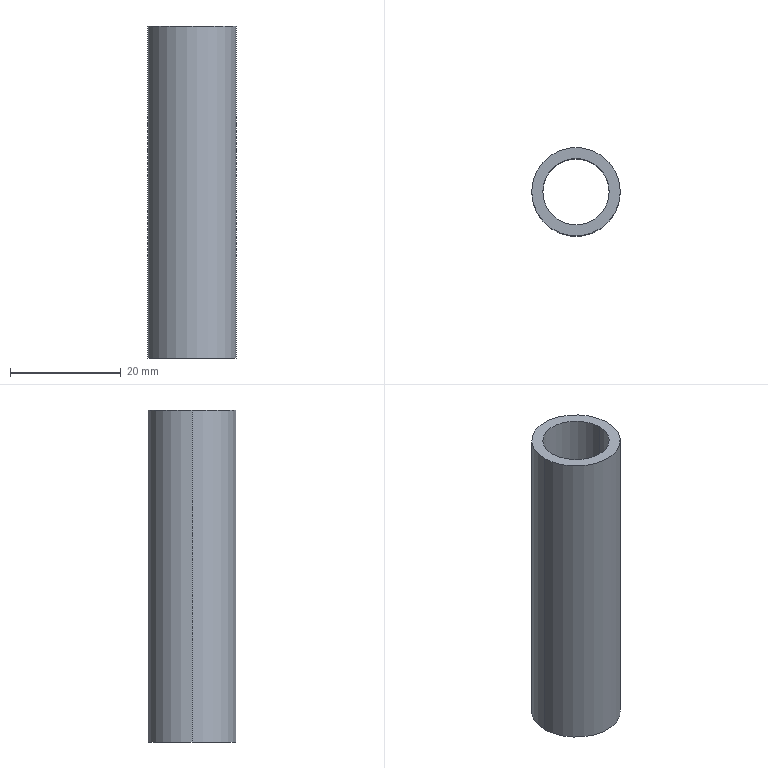Part | SolidWorks | features Extrusion 1 | 1 solid | 6 faces | box 16 x 16 x 60 mm | volume 5278 mm3 | cylinder 4 | plane 2 | commonest cylinder face diameters 12 x2 16 x2
STEP:
#1=CARTESIAN_POINT('',(-6.,0.,60.));
#2=VERTEX_POINT('',#1);
#3=CARTESIAN_POINT('',(6.,0.,60.));
#4=VERTEX_POINT('',#3);
#5=CARTESIAN_POINT('',(0.,0.,60.));
#6=DIRECTION('',(0.,0.,1.));
#7=DIRECTION('',(1.,0.,0.));
#8=AXIS2_PLACEMENT_3D('',#5,#6,#7);
#9=CIRCLE('',#8,6.);
#10=EDGE_CURVE('',#2,#4,#9,.T.);
#11=ORIENTED_EDGE('',*,*,#10,.T.);
#12=CARTESIAN_POINT('',(6.,0.,0.));
#13=VERTEX_POINT('',#12);
#14=CARTESIAN_POINT('',(6.,0.,60.));
#15=DIRECTION('',(0.,0.,-1.));
#16=VECTOR('',#15,1000.);
#17=LINE('',#14,#16);
#18=EDGE_CURVE('',#4,#13,#17,.T.);
#19=ORIENTED_EDGE('',*,*,#18,.T.);
#20=CARTESIAN_POINT('',(-6.,0.,0.));
#21=VERTEX_POINT('',#20);
#22=CARTESIAN_POINT('',(0.,0.,0.));
#23=DIRECTION('',(0.,0.,1.));
#24=DIRECTION('',(1.,0.,0.));
#25=AXIS2_PLACEMENT_3D('',#22,#23,#24);
#26=CIRCLE('',#25,6.);
#27=EDGE_CURVE('',#21,#13,#26,.T.);
#28=ORIENTED_EDGE('',*,*,#27,.F.);
#29=CARTESIAN_POINT('',(-6.,0.,60.));
#30=DIRECTION('',(0.,0.,-1.));
#31=VECTOR('',#30,1000.);
#32=LINE('',#29,#31);
#33=EDGE_CURVE('',#2,#21,#32,.T.);
#34=ORIENTED_EDGE('',*,*,#33,.F.);
#35=EDGE_LOOP('',(#11,#19,#28,#34));
#36=FACE_OUTER_BOUND('',#35,.T.);
#37=CARTESIAN_POINT('',(0.,0.,60.));
#38=DIRECTION('',(0.,0.,-1.));
#39=DIRECTION('',(-1.,0.,0.));
#40=AXIS2_PLACEMENT_3D('',#37,#38,#39);
#41=CYLINDRICAL_SURFACE('',#40,6.);
#42=ADVANCED_FACE('',(#36),#41,.F.);
#43=CARTESIAN_POINT('',(8.,0.,60.));
#44=VERTEX_POINT('',#43);
#45=CARTESIAN_POINT('',(-8.,0.,60.));
#46=VERTEX_POINT('',#45);
#47=CARTESIAN_POINT('',(0.,0.,60.));
#48=DIRECTION('',(0.,0.,1.));
#49=DIRECTION('',(1.,0.,0.));
#50=AXIS2_PLACEMENT_3D('',#47,#48,#49);
#51=CIRCLE('',#50,8.);
#52=EDGE_CURVE('',#44,#46,#51,.T.);
#53=ORIENTED_EDGE('',*,*,#52,.F.);
#54=CARTESIAN_POINT('',(8.,0.,0.));
#55=VERTEX_POINT('',#54);
#56=CARTESIAN_POINT('',(8.,0.,60.));
#57=DIRECTION('',(0.,0.,-1.));
#58=VECTOR('',#57,1000.);
#59=LINE('',#56,#58);
#60=EDGE_CURVE('',#44,#55,#59,.T.);
#61=ORIENTED_EDGE('',*,*,#60,.T.);
#62=CARTESIAN_POINT('',(-8.,0.,0.));
#63=VERTEX_POINT('',#62);
#64=CARTESIAN_POINT('',(0.,0.,0.));
#65=DIRECTION('',(0.,0.,1.));
#66=DIRECTION('',(1.,0.,0.));
#67=AXIS2_PLACEMENT_3D('',#64,#65,#66);
#68=CIRCLE('',#67,8.);
#69=EDGE_CURVE('',#55,#63,#68,.T.);
#70=ORIENTED_EDGE('',*,*,#69,.T.);
#71=CARTESIAN_POINT('',(-8.,0.,60.));
#72=DIRECTION('',(0.,0.,-1.));
#73=VECTOR('',#72,1000.);
#74=LINE('',#71,#73);
#75=EDGE_CURVE('',#46,#63,#74,.T.);
#76=ORIENTED_EDGE('',*,*,#75,.F.);
#77=EDGE_LOOP('',(#53,#61,#70,#76));
#78=FACE_OUTER_BOUND('',#77,.T.);
#79=CARTESIAN_POINT('',(0.,0.,60.));
#80=DIRECTION('',(0.,0.,-1.));
#81=DIRECTION('',(-1.,0.,0.));
#82=AXIS2_PLACEMENT_3D('',#79,#80,#81);
#83=CYLINDRICAL_SURFACE('',#82,8.);
#84=ADVANCED_FACE('',(#78),#83,.T.);
#85=CARTESIAN_POINT('',(0.,0.,60.));
#86=DIRECTION('',(0.,0.,1.));
#87=DIRECTION('',(1.,0.,0.));
#88=AXIS2_PLACEMENT_3D('',#85,#86,#87);
#89=CIRCLE('',#88,8.);
#90=EDGE_CURVE('',#46,#44,#89,.T.);
#91=ORIENTED_EDGE('',*,*,#90,.T.);
#92=ORIENTED_EDGE('',*,*,#52,.T.);
#93=EDGE_LOOP('',(#91,#92));
#94=FACE_OUTER_BOUND('',#93,.T.);
#95=ORIENTED_EDGE('',*,*,#10,.F.);
#96=CARTESIAN_POINT('',(0.,0.,60.));
#97=DIRECTION('',(0.,0.,1.));
#98=DIRECTION('',(1.,0.,0.));
#99=AXIS2_PLACEMENT_3D('',#96,#97,#98);
#100=CIRCLE('',#99,6.);
#101=EDGE_CURVE('',#4,#2,#100,.T.);
#102=ORIENTED_EDGE('',*,*,#101,.F.);
#103=EDGE_LOOP('',(#95,#102));
#104=FACE_BOUND('',#103,.T.);
#105=CARTESIAN_POINT('',(0.,0.,60.));
#106=DIRECTION('',(0.,0.,1.));
#107=DIRECTION('',(1.,0.,0.));
#108=AXIS2_PLACEMENT_3D('',#105,#106,#107);
#109=PLANE('',#108);
#110=ADVANCED_FACE('',(#94,#104),#109,.T.);
#111=CARTESIAN_POINT('',(0.,0.,0.));
#112=DIRECTION('',(0.,0.,1.));
#113=DIRECTION('',(1.,0.,0.));
#114=AXIS2_PLACEMENT_3D('',#111,#112,#113);
#115=CIRCLE('',#114,8.);
#116=EDGE_CURVE('',#63,#55,#115,.T.);
#117=ORIENTED_EDGE('',*,*,#116,.F.);
#118=ORIENTED_EDGE('',*,*,#69,.F.);
#119=EDGE_LOOP('',(#117,#118));
#120=FACE_OUTER_BOUND('',#119,.T.);
#121=ORIENTED_EDGE('',*,*,#27,.T.);
#122=CARTESIAN_POINT('',(0.,0.,0.));
#123=DIRECTION('',(0.,0.,1.));
#124=DIRECTION('',(1.,0.,0.));
#125=AXIS2_PLACEMENT_3D('',#122,#123,#124);
#126=CIRCLE('',#125,6.);
#127=EDGE_CURVE('',#13,#21,#126,.T.);
#128=ORIENTED_EDGE('',*,*,#127,.T.);
#129=EDGE_LOOP('',(#121,#128));
#130=FACE_BOUND('',#129,.T.);
#131=CARTESIAN_POINT('',(0.,0.,0.));
#132=DIRECTION('',(0.,0.,1.));
#133=DIRECTION('',(1.,0.,0.));
#134=AXIS2_PLACEMENT_3D('',#131,#132,#133);
#135=PLANE('',#134);
#136=ADVANCED_FACE('',(#120,#130),#135,.F.);
#137=ORIENTED_EDGE('',*,*,#60,.F.);
#138=ORIENTED_EDGE('',*,*,#90,.F.);
#139=ORIENTED_EDGE('',*,*,#75,.T.);
#140=ORIENTED_EDGE('',*,*,#116,.T.);
#141=EDGE_LOOP('',(#137,#138,#139,#140));
#142=FACE_OUTER_BOUND('',#141,.T.);
#143=CARTESIAN_POINT('',(0.,0.,60.));
#144=DIRECTION('',(0.,0.,-1.));
#145=DIRECTION('',(-1.,0.,0.));
#146=AXIS2_PLACEMENT_3D('',#143,#144,#145);
#147=CYLINDRICAL_SURFACE('',#146,8.);
#148=ADVANCED_FACE('',(#142),#147,.T.);
#149=ORIENTED_EDGE('',*,*,#18,.F.);
#150=ORIENTED_EDGE('',*,*,#101,.T.);
#151=ORIENTED_EDGE('',*,*,#33,.T.);
#152=ORIENTED_EDGE('',*,*,#127,.F.);
#153=EDGE_LOOP('',(#149,#150,#151,#152));
#154=FACE_OUTER_BOUND('',#153,.T.);
#155=CARTESIAN_POINT('',(0.,0.,60.));
#156=DIRECTION('',(0.,0.,-1.));
#157=DIRECTION('',(-1.,0.,0.));
#158=AXIS2_PLACEMENT_3D('',#155,#156,#157);
#159=CYLINDRICAL_SURFACE('',#158,6.);
#160=ADVANCED_FACE('',(#154),#159,.F.);
#161=CLOSED_SHELL('',(#42,#84,#110,#136,#148,#160));
#162=MANIFOLD_SOLID_BREP('',#161);
#163=CARTESIAN_POINT('',(0.,0.,0.));
#164=DIRECTION('',(0.,0.,1.));
#165=DIRECTION('',(1.,0.,0.));
#166=AXIS2_PLACEMENT_3D('',#163,#164,#165);
#167=(LENGTH_UNIT()NAMED_UNIT(*)SI_UNIT(.MILLI.,.METRE.));
#168=UNCERTAINTY_MEASURE_WITH_UNIT(LENGTH_MEASURE(0.00001),#167,'','');
#169=(NAMED_UNIT(*)PLANE_ANGLE_UNIT()SI_UNIT($,.RADIAN.));
#170=(NAMED_UNIT(*)SI_UNIT($,.STERADIAN.)SOLID_ANGLE_UNIT());
#171=(GEOMETRIC_REPRESENTATION_CONTEXT(3)GLOBAL_UNCERTAINTY_ASSIGNED_CONTEXT((#168))GLOBAL_UNIT_ASSIGNED_CONTEXT((#167,#169,#170))REPRESENTATION_CONTEXT('',''));
#172=ADVANCED_BREP_SHAPE_REPRESENTATION('',(#162,#166),#171);